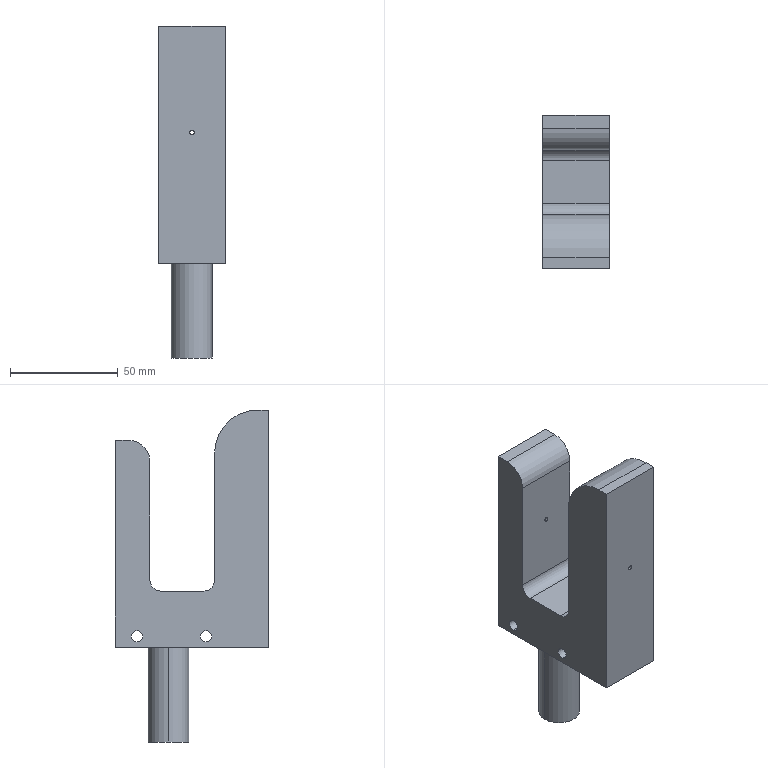Part | SolidWorks | features Fillet 3, HoleWzd 2, ICE 2, Extrusion 1 | 1 solid | 29 faces | box 31 x 71 x 154 mm | volume 164742 mm3 | cylinder 16 | plane 11 | cone 2 | commonest cylinder face diameters 2 x4 5.2 x4 5 x2 10 x2 18.868 x2 20 x1
STEP:
#1=CARTESIAN_POINT('',(5.937,16.378,-84.621));
#2=VERTEX_POINT('',#1);
#3=CARTESIAN_POINT('',(24.805,16.378,-84.621));
#4=VERTEX_POINT('',#3);
#5=CARTESIAN_POINT('',(15.371,16.378,-84.621));
#6=DIRECTION('',(0.,0.,-1.));
#7=DIRECTION('',(-1.,0.,0.));
#8=AXIS2_PLACEMENT_3D('',#5,#6,#7);
#9=CIRCLE('',#8,9.434);
#10=EDGE_CURVE('',#2,#4,#9,.T.);
#11=ORIENTED_EDGE('',*,*,#10,.F.);
#12=CARTESIAN_POINT('',(5.937,16.378,-40.621));
#13=VERTEX_POINT('',#12);
#14=CARTESIAN_POINT('',(5.937,16.378,-84.621));
#15=DIRECTION('',(0.,0.,1.));
#16=VECTOR('',#15,1000.);
#17=LINE('',#14,#16);
#18=EDGE_CURVE('',#2,#13,#17,.T.);
#19=ORIENTED_EDGE('',*,*,#18,.T.);
#20=CARTESIAN_POINT('',(24.805,16.378,-40.621));
#21=VERTEX_POINT('',#20);
#22=CARTESIAN_POINT('',(15.371,16.378,-40.621));
#23=DIRECTION('',(0.,0.,-1.));
#24=DIRECTION('',(1.,0.,0.));
#25=AXIS2_PLACEMENT_3D('',#22,#23,#24);
#26=CIRCLE('',#25,9.434);
#27=EDGE_CURVE('',#13,#21,#26,.T.);
#28=ORIENTED_EDGE('',*,*,#27,.T.);
#29=CARTESIAN_POINT('',(24.805,16.378,-84.621));
#30=DIRECTION('',(0.,0.,1.));
#31=VECTOR('',#30,1000.);
#32=LINE('',#29,#31);
#33=EDGE_CURVE('',#4,#21,#32,.T.);
#34=ORIENTED_EDGE('',*,*,#33,.F.);
#35=EDGE_LOOP('',(#11,#19,#28,#34));
#36=FACE_OUTER_BOUND('',#35,.T.);
#37=CARTESIAN_POINT('',(15.371,16.378,-84.621));
#38=DIRECTION('',(0.,0.,1.));
#39=DIRECTION('',(1.,0.,0.));
#40=AXIS2_PLACEMENT_3D('',#37,#38,#39);
#41=CYLINDRICAL_SURFACE('',#40,9.434);
#42=ADVANCED_FACE('',(#36),#41,.T.);
#43=CARTESIAN_POINT('',(18.,-13.042,-32.621));
#44=VERTEX_POINT('',#43);
#45=CARTESIAN_POINT('',(13.,-13.042,-32.621));
#46=VERTEX_POINT('',#45);
#47=CARTESIAN_POINT('',(15.5,-13.042,-32.621));
#48=DIRECTION('',(0.,0.,-1.));
#49=DIRECTION('',(-1.,0.,0.));
#50=AXIS2_PLACEMENT_3D('',#47,#48,#49);
#51=CIRCLE('',#50,2.5);
#52=EDGE_CURVE('',#44,#46,#51,.T.);
#53=ORIENTED_EDGE('',*,*,#52,.F.);
#54=CARTESIAN_POINT('',(18.,-13.042,-40.621));
#55=VERTEX_POINT('',#54);
#56=CARTESIAN_POINT('',(18.,-13.042,-40.621));
#57=DIRECTION('',(0.,0.,-1.));
#58=VECTOR('',#57,1000.);
#59=LINE('',#56,#58);
#60=EDGE_CURVE('',#44,#55,#59,.T.);
#61=ORIENTED_EDGE('',*,*,#60,.T.);
#62=CARTESIAN_POINT('',(13.,-13.042,-40.621));
#63=VERTEX_POINT('',#62);
#64=CARTESIAN_POINT('',(15.5,-13.042,-40.621));
#65=DIRECTION('',(0.,0.,-1.));
#66=DIRECTION('',(-1.,0.,0.));
#67=AXIS2_PLACEMENT_3D('',#64,#65,#66);
#68=CIRCLE('',#67,2.5);
#69=EDGE_CURVE('',#55,#63,#68,.T.);
#70=ORIENTED_EDGE('',*,*,#69,.T.);
#71=CARTESIAN_POINT('',(13.,-13.042,-40.621));
#72=DIRECTION('',(0.,0.,-1.));
#73=VECTOR('',#72,1000.);
#74=LINE('',#71,#73);
#75=EDGE_CURVE('',#46,#63,#74,.T.);
#76=ORIENTED_EDGE('',*,*,#75,.F.);
#77=EDGE_LOOP('',(#53,#61,#70,#76));
#78=FACE_OUTER_BOUND('',#77,.T.);
#79=CARTESIAN_POINT('',(15.5,-13.042,-40.621));
#80=DIRECTION('',(0.,0.,-1.));
#81=DIRECTION('',(-1.,0.,0.));
#82=AXIS2_PLACEMENT_3D('',#79,#80,#81);
#83=CYLINDRICAL_SURFACE('',#82,2.5);
#84=ADVANCED_FACE('',(#78),#83,.F.);
#85=CARTESIAN_POINT('',(15.5,-13.042,-31.119));
#86=VERTEX_POINT('',#85);
#87=CARTESIAN_POINT('',(13.,-13.042,-32.621));
#88=DIRECTION('',(-0.8572,0.,-0.515));
#89=VECTOR('',#88,1000.);
#90=LINE('',#87,#89);
#91=EDGE_CURVE('',#86,#46,#90,.T.);
#92=ORIENTED_EDGE('',*,*,#91,.F.);
#93=CARTESIAN_POINT('',(18.,-13.042,-32.621));
#94=DIRECTION('',(0.8572,0.,-0.515));
#95=VECTOR('',#94,1000.);
#96=LINE('',#93,#95);
#97=EDGE_CURVE('',#86,#44,#96,.T.);
#98=ORIENTED_EDGE('',*,*,#97,.T.);
#99=ORIENTED_EDGE('',*,*,#52,.T.);
#100=EDGE_LOOP('',(#92,#98,#99));
#101=FACE_OUTER_BOUND('',#100,.T.);
#102=CARTESIAN_POINT('',(15.5,-13.042,-32.621));
#103=DIRECTION('',(0.,0.,-1.));
#104=DIRECTION('',(-1.,0.,0.));
#105=AXIS2_PLACEMENT_3D('',#102,#103,#104);
#106=CONICAL_SURFACE('',#105,2.5,1.03);
#107=ADVANCED_FACE('',(#101),#106,.F.);
#108=CARTESIAN_POINT('',(0.,30.958,-33.021));
#109=VERTEX_POINT('',#108);
#110=CARTESIAN_POINT('',(0.,30.958,-38.221));
#111=VERTEX_POINT('',#110);
#112=CARTESIAN_POINT('',(0.,30.958,-35.621));
#113=DIRECTION('',(1.,0.,0.));
#114=DIRECTION('',(0.,0.,-1.));
#115=AXIS2_PLACEMENT_3D('',#112,#113,#114);
#116=CIRCLE('',#115,2.6);
#117=EDGE_CURVE('',#109,#111,#116,.T.);
#118=ORIENTED_EDGE('',*,*,#117,.F.);
#119=CARTESIAN_POINT('',(31.,30.958,-33.021));
#120=VERTEX_POINT('',#119);
#121=CARTESIAN_POINT('',(31.,30.958,-33.021));
#122=DIRECTION('',(1.,0.,0.));
#123=VECTOR('',#122,1000.);
#124=LINE('',#121,#123);
#125=EDGE_CURVE('',#109,#120,#124,.T.);
#126=ORIENTED_EDGE('',*,*,#125,.T.);
#127=CARTESIAN_POINT('',(31.,30.958,-38.221));
#128=VERTEX_POINT('',#127);
#129=CARTESIAN_POINT('',(31.,30.958,-35.621));
#130=DIRECTION('',(1.,0.,0.));
#131=DIRECTION('',(0.,0.,-1.));
#132=AXIS2_PLACEMENT_3D('',#129,#130,#131);
#133=CIRCLE('',#132,2.6);
#134=EDGE_CURVE('',#120,#128,#133,.T.);
#135=ORIENTED_EDGE('',*,*,#134,.T.);
#136=CARTESIAN_POINT('',(31.,30.958,-38.221));
#137=DIRECTION('',(1.,0.,0.));
#138=VECTOR('',#137,1000.);
#139=LINE('',#136,#138);
#140=EDGE_CURVE('',#111,#128,#139,.T.);
#141=ORIENTED_EDGE('',*,*,#140,.F.);
#142=EDGE_LOOP('',(#118,#126,#135,#141));
#143=FACE_OUTER_BOUND('',#142,.T.);
#144=CARTESIAN_POINT('',(31.,30.958,-35.621));
#145=DIRECTION('',(1.,0.,0.));
#146=DIRECTION('',(0.,0.,-1.));
#147=AXIS2_PLACEMENT_3D('',#144,#145,#146);
#148=CYLINDRICAL_SURFACE('',#147,2.6);
#149=ADVANCED_FACE('',(#143),#148,.F.);
#150=CARTESIAN_POINT('',(0.,-1.042,-33.021));
#151=VERTEX_POINT('',#150);
#152=CARTESIAN_POINT('',(0.,-1.042,-38.221));
#153=VERTEX_POINT('',#152);
#154=CARTESIAN_POINT('',(0.,-1.042,-35.621));
#155=DIRECTION('',(1.,0.,0.));
#156=DIRECTION('',(0.,0.,-1.));
#157=AXIS2_PLACEMENT_3D('',#154,#155,#156);
#158=CIRCLE('',#157,2.6);
#159=EDGE_CURVE('',#151,#153,#158,.T.);
#160=ORIENTED_EDGE('',*,*,#159,.F.);
#161=CARTESIAN_POINT('',(31.,-1.042,-33.021));
#162=VERTEX_POINT('',#161);
#163=CARTESIAN_POINT('',(31.,-1.042,-33.021));
#164=DIRECTION('',(1.,0.,0.));
#165=VECTOR('',#164,1000.);
#166=LINE('',#163,#165);
#167=EDGE_CURVE('',#151,#162,#166,.T.);
#168=ORIENTED_EDGE('',*,*,#167,.T.);
#169=CARTESIAN_POINT('',(31.,-1.042,-38.221));
#170=VERTEX_POINT('',#169);
#171=CARTESIAN_POINT('',(31.,-1.042,-35.621));
#172=DIRECTION('',(1.,0.,0.));
#173=DIRECTION('',(0.,0.,-1.));
#174=AXIS2_PLACEMENT_3D('',#171,#172,#173);
#175=CIRCLE('',#174,2.6);
#176=EDGE_CURVE('',#162,#170,#175,.T.);
#177=ORIENTED_EDGE('',*,*,#176,.T.);
#178=CARTESIAN_POINT('',(31.,-1.042,-38.221));
#179=DIRECTION('',(1.,0.,0.));
#180=VECTOR('',#179,1000.);
#181=LINE('',#178,#180);
#182=EDGE_CURVE('',#153,#170,#181,.T.);
#183=ORIENTED_EDGE('',*,*,#182,.F.);
#184=EDGE_LOOP('',(#160,#168,#177,#183));
#185=FACE_OUTER_BOUND('',#184,.T.);
#186=CARTESIAN_POINT('',(31.,-1.042,-35.621));
#187=DIRECTION('',(1.,0.,0.));
#188=DIRECTION('',(0.,0.,-1.));
#189=AXIS2_PLACEMENT_3D('',#186,#187,#188);
#190=CYLINDRICAL_SURFACE('',#189,2.6);
#191=ADVANCED_FACE('',(#185),#190,.F.);
#192=CARTESIAN_POINT('',(15.5,24.958,18.879));
#193=VERTEX_POINT('',#192);
#194=CARTESIAN_POINT('',(15.5,24.958,20.879));
#195=VERTEX_POINT('',#194);
#196=CARTESIAN_POINT('',(15.5,24.958,19.879));
#197=DIRECTION('',(0.,1.,0.));
#198=DIRECTION('',(0.,0.,1.));
#199=AXIS2_PLACEMENT_3D('',#196,#197,#198);
#200=CIRCLE('',#199,1.);
#201=EDGE_CURVE('',#193,#195,#200,.T.);
#202=ORIENTED_EDGE('',*,*,#201,.F.);
#203=CARTESIAN_POINT('',(15.5,40.958,18.879));
#204=VERTEX_POINT('',#203);
#205=CARTESIAN_POINT('',(15.5,-30.042,18.879));
#206=DIRECTION('',(0.,1.,0.));
#207=VECTOR('',#206,1000.);
#208=LINE('',#205,#207);
#209=EDGE_CURVE('',#193,#204,#208,.T.);
#210=ORIENTED_EDGE('',*,*,#209,.T.);
#211=CARTESIAN_POINT('',(15.5,40.958,20.879));
#212=VERTEX_POINT('',#211);
#213=CARTESIAN_POINT('',(15.5,40.958,19.879));
#214=DIRECTION('',(0.,1.,0.));
#215=DIRECTION('',(0.,0.,1.));
#216=AXIS2_PLACEMENT_3D('',#213,#214,#215);
#217=CIRCLE('',#216,1.);
#218=EDGE_CURVE('',#204,#212,#217,.T.);
#219=ORIENTED_EDGE('',*,*,#218,.T.);
#220=CARTESIAN_POINT('',(15.5,-30.042,20.879));
#221=DIRECTION('',(0.,1.,0.));
#222=VECTOR('',#221,1000.);
#223=LINE('',#220,#222);
#224=EDGE_CURVE('',#195,#212,#223,.T.);
#225=ORIENTED_EDGE('',*,*,#224,.F.);
#226=EDGE_LOOP('',(#202,#210,#219,#225));
#227=FACE_OUTER_BOUND('',#226,.T.);
#228=CARTESIAN_POINT('',(15.5,-30.042,19.879));
#229=DIRECTION('',(0.,1.,0.));
#230=DIRECTION('',(0.,0.,1.));
#231=AXIS2_PLACEMENT_3D('',#228,#229,#230);
#232=CYLINDRICAL_SURFACE('',#231,1.);
#233=ADVANCED_FACE('',(#227),#232,.F.);
#234=CARTESIAN_POINT('',(15.5,-30.042,18.879));
#235=VERTEX_POINT('',#234);
#236=CARTESIAN_POINT('',(15.5,-30.042,20.879));
#237=VERTEX_POINT('',#236);
#238=CARTESIAN_POINT('',(15.5,-30.042,19.879));
#239=DIRECTION('',(0.,1.,0.));
#240=DIRECTION('',(0.,0.,1.));
#241=AXIS2_PLACEMENT_3D('',#238,#239,#240);
#242=CIRCLE('',#241,1.);
#243=EDGE_CURVE('',#235,#237,#242,.T.);
#244=ORIENTED_EDGE('',*,*,#243,.F.);
#245=CARTESIAN_POINT('',(15.5,-5.042,18.879));
#246=VERTEX_POINT('',#245);
#247=CARTESIAN_POINT('',(15.5,-30.042,18.879));
#248=DIRECTION('',(0.,1.,0.));
#249=VECTOR('',#248,1000.);
#250=LINE('',#247,#249);
#251=EDGE_CURVE('',#235,#246,#250,.T.);
#252=ORIENTED_EDGE('',*,*,#251,.T.);
#253=CARTESIAN_POINT('',(15.5,-5.042,20.879));
#254=VERTEX_POINT('',#253);
#255=CARTESIAN_POINT('',(15.5,-5.042,19.879));
#256=DIRECTION('',(0.,-1.,0.));
#257=DIRECTION('',(0.,0.,-1.));
#258=AXIS2_PLACEMENT_3D('',#255,#256,#257);
#259=CIRCLE('',#258,1.);
#260=EDGE_CURVE('',#254,#246,#259,.T.);
#261=ORIENTED_EDGE('',*,*,#260,.F.);
#262=CARTESIAN_POINT('',(15.5,-30.042,20.879));
#263=DIRECTION('',(0.,1.,0.));
#264=VECTOR('',#263,1000.);
#265=LINE('',#262,#264);
#266=EDGE_CURVE('',#237,#254,#265,.T.);
#267=ORIENTED_EDGE('',*,*,#266,.F.);
#268=EDGE_LOOP('',(#244,#252,#261,#267));
#269=FACE_OUTER_BOUND('',#268,.T.);
#270=CARTESIAN_POINT('',(15.5,-30.042,19.879));
#271=DIRECTION('',(0.,1.,0.));
#272=DIRECTION('',(0.,0.,1.));
#273=AXIS2_PLACEMENT_3D('',#270,#271,#272);
#274=CYLINDRICAL_SURFACE('',#273,1.);
#275=ADVANCED_FACE('',(#269),#274,.F.);
#276=CARTESIAN_POINT('',(15.371,16.378,-40.621));
#277=DIRECTION('',(0.,0.,-1.));
#278=DIRECTION('',(1.,0.,0.));
#279=AXIS2_PLACEMENT_3D('',#276,#277,#278);
#280=CIRCLE('',#279,9.434);
#281=EDGE_CURVE('',#21,#13,#280,.T.);
#282=ORIENTED_EDGE('',*,*,#281,.F.);
#283=ORIENTED_EDGE('',*,*,#27,.F.);
#284=EDGE_LOOP('',(#282,#283));
#285=FACE_BOUND('',#284,.T.);
#286=CARTESIAN_POINT('',(15.5,-13.042,-40.621));
#287=DIRECTION('',(0.,0.,-1.));
#288=DIRECTION('',(-1.,0.,0.));
#289=AXIS2_PLACEMENT_3D('',#286,#287,#288);
#290=CIRCLE('',#289,2.5);
#291=EDGE_CURVE('',#63,#55,#290,.T.);
#292=ORIENTED_EDGE('',*,*,#291,.F.);
#293=ORIENTED_EDGE('',*,*,#69,.F.);
#294=EDGE_LOOP('',(#292,#293));
#295=FACE_BOUND('',#294,.T.);
#296=CARTESIAN_POINT('',(0.,-30.042,-40.621));
#297=VERTEX_POINT('',#296);
#298=CARTESIAN_POINT('',(0.,40.958,-40.621));
#299=VERTEX_POINT('',#298);
#300=CARTESIAN_POINT('',(0.,40.958,-40.621));
#301=DIRECTION('',(0.,1.,0.));
#302=VECTOR('',#301,1000.);
#303=LINE('',#300,#302);
#304=EDGE_CURVE('',#297,#299,#303,.T.);
#305=ORIENTED_EDGE('',*,*,#304,.T.);
#306=CARTESIAN_POINT('',(31.,40.958,-40.621));
#307=VERTEX_POINT('',#306);
#308=CARTESIAN_POINT('',(31.,40.958,-40.621));
#309=DIRECTION('',(-1.,0.,0.));
#310=VECTOR('',#309,1000.);
#311=LINE('',#308,#310);
#312=EDGE_CURVE('',#307,#299,#311,.T.);
#313=ORIENTED_EDGE('',*,*,#312,.F.);
#314=CARTESIAN_POINT('',(31.,-30.042,-40.621));
#315=VERTEX_POINT('',#314);
#316=CARTESIAN_POINT('',(31.,40.958,-40.621));
#317=DIRECTION('',(0.,1.,0.));
#318=VECTOR('',#317,1000.);
#319=LINE('',#316,#318);
#320=EDGE_CURVE('',#315,#307,#319,.T.);
#321=ORIENTED_EDGE('',*,*,#320,.F.);
#322=CARTESIAN_POINT('',(31.,-30.042,-40.621));
#323=DIRECTION('',(-1.,0.,0.));
#324=VECTOR('',#323,1000.);
#325=LINE('',#322,#324);
#326=EDGE_CURVE('',#315,#297,#325,.T.);
#327=ORIENTED_EDGE('',*,*,#326,.T.);
#328=EDGE_LOOP('',(#305,#313,#321,#327));
#329=FACE_OUTER_BOUND('',#328,.T.);
#330=CARTESIAN_POINT('',(31.,40.958,-40.621));
#331=DIRECTION('',(0.,0.,1.));
#332=DIRECTION('',(1.,0.,0.));
#333=AXIS2_PLACEMENT_3D('',#330,#331,#332);
#334=PLANE('',#333);
#335=ADVANCED_FACE('',(#285,#295,#329),#334,.F.);
#336=CARTESIAN_POINT('',(15.5,40.958,19.879));
#337=DIRECTION('',(0.,1.,0.));
#338=DIRECTION('',(0.,0.,1.));
#339=AXIS2_PLACEMENT_3D('',#336,#337,#338);
#340=CIRCLE('',#339,1.);
#341=EDGE_CURVE('',#212,#204,#340,.T.);
#342=ORIENTED_EDGE('',*,*,#341,.F.);
#343=ORIENTED_EDGE('',*,*,#218,.F.);
#344=EDGE_LOOP('',(#342,#343));
#345=FACE_BOUND('',#344,.T.);
#346=CARTESIAN_POINT('',(0.,40.958,55.379));
#347=VERTEX_POINT('',#346);
#348=CARTESIAN_POINT('',(0.,40.958,55.379));
#349=DIRECTION('',(0.,0.,1.));
#350=VECTOR('',#349,1000.);
#351=LINE('',#348,#350);
#352=EDGE_CURVE('',#299,#347,#351,.T.);
#353=ORIENTED_EDGE('',*,*,#352,.T.);
#354=CARTESIAN_POINT('',(31.,40.958,55.379));
#355=VERTEX_POINT('',#354);
#356=CARTESIAN_POINT('',(31.,40.958,55.379));
#357=DIRECTION('',(-1.,0.,0.));
#358=VECTOR('',#357,1000.);
#359=LINE('',#356,#358);
#360=EDGE_CURVE('',#355,#347,#359,.T.);
#361=ORIENTED_EDGE('',*,*,#360,.F.);
#362=CARTESIAN_POINT('',(31.,40.958,55.379));
#363=DIRECTION('',(0.,0.,1.));
#364=VECTOR('',#363,1000.);
#365=LINE('',#362,#364);
#366=EDGE_CURVE('',#307,#355,#365,.T.);
#367=ORIENTED_EDGE('',*,*,#366,.F.);
#368=ORIENTED_EDGE('',*,*,#312,.T.);
#369=EDGE_LOOP('',(#353,#361,#367,#368));
#370=FACE_OUTER_BOUND('',#369,.T.);
#371=CARTESIAN_POINT('',(31.,40.958,55.379));
#372=DIRECTION('',(0.,-1.,0.));
#373=DIRECTION('',(0.,0.,-1.));
#374=AXIS2_PLACEMENT_3D('',#371,#372,#373);
#375=PLANE('',#374);
#376=ADVANCED_FACE('',(#345,#370),#375,.F.);
#377=CARTESIAN_POINT('',(0.,34.958,55.379));
#378=VERTEX_POINT('',#377);
#379=CARTESIAN_POINT('',(0.,40.958,55.379));
#380=DIRECTION('',(0.,-1.,0.));
#381=VECTOR('',#380,1000.);
#382=LINE('',#379,#381);
#383=EDGE_CURVE('',#347,#378,#382,.T.);
#384=ORIENTED_EDGE('',*,*,#383,.T.);
#385=CARTESIAN_POINT('',(31.,34.958,55.379));
#386=VERTEX_POINT('',#385);
#387=CARTESIAN_POINT('',(31.,34.958,55.379));
#388=DIRECTION('',(1.,0.,0.));
#389=VECTOR('',#388,1000.);
#390=LINE('',#387,#389);
#391=EDGE_CURVE('',#378,#386,#390,.T.);
#392=ORIENTED_EDGE('',*,*,#391,.T.);
#393=CARTESIAN_POINT('',(31.,40.958,55.379));
#394=DIRECTION('',(0.,-1.,0.));
#395=VECTOR('',#394,1000.);
#396=LINE('',#393,#395);
#397=EDGE_CURVE('',#355,#386,#396,.T.);
#398=ORIENTED_EDGE('',*,*,#397,.F.);
#399=ORIENTED_EDGE('',*,*,#360,.T.);
#400=EDGE_LOOP('',(#384,#392,#398,#399));
#401=FACE_OUTER_BOUND('',#400,.T.);
#402=CARTESIAN_POINT('',(31.,40.958,55.379));
#403=DIRECTION('',(0.,0.,-1.));
#404=DIRECTION('',(-1.,0.,0.));
#405=AXIS2_PLACEMENT_3D('',#402,#403,#404);
#406=PLANE('',#405);
#407=ADVANCED_FACE('',(#401),#406,.F.);
#408=CARTESIAN_POINT('',(15.5,24.958,19.879));
#409=DIRECTION('',(0.,1.,0.));
#410=DIRECTION('',(0.,0.,1.));
#411=AXIS2_PLACEMENT_3D('',#408,#409,#410);
#412=CIRCLE('',#411,1.);
#413=EDGE_CURVE('',#195,#193,#412,.T.);
#414=ORIENTED_EDGE('',*,*,#413,.T.);
#415=ORIENTED_EDGE('',*,*,#201,.T.);
#416=EDGE_LOOP('',(#414,#415));
#417=FACE_BOUND('',#416,.T.);
#418=CARTESIAN_POINT('',(0.,24.958,45.379));
#419=VERTEX_POINT('',#418);
#420=CARTESIAN_POINT('',(0.,24.958,-9.621));
#421=VERTEX_POINT('',#420);
#422=CARTESIAN_POINT('',(0.,24.958,55.379));
#423=DIRECTION('',(0.,0.,-1.));
#424=VECTOR('',#423,1000.);
#425=LINE('',#422,#424);
#426=EDGE_CURVE('',#419,#421,#425,.T.);
#427=ORIENTED_EDGE('',*,*,#426,.T.);
#428=CARTESIAN_POINT('',(31.,24.958,-9.621));
#429=VERTEX_POINT('',#428);
#430=CARTESIAN_POINT('',(31.,24.958,-9.621));
#431=DIRECTION('',(1.,0.,0.));
#432=VECTOR('',#431,1000.);
#433=LINE('',#430,#432);
#434=EDGE_CURVE('',#421,#429,#433,.T.);
#435=ORIENTED_EDGE('',*,*,#434,.T.);
#436=CARTESIAN_POINT('',(31.,24.958,45.379));
#437=VERTEX_POINT('',#436);
#438=CARTESIAN_POINT('',(31.,24.958,55.379));
#439=DIRECTION('',(0.,0.,-1.));
#440=VECTOR('',#439,1000.);
#441=LINE('',#438,#440);
#442=EDGE_CURVE('',#437,#429,#441,.T.);
#443=ORIENTED_EDGE('',*,*,#442,.F.);
#444=CARTESIAN_POINT('',(31.,24.958,45.379));
#445=DIRECTION('',(-1.,0.,0.));
#446=VECTOR('',#445,1000.);
#447=LINE('',#444,#446);
#448=EDGE_CURVE('',#437,#419,#447,.T.);
#449=ORIENTED_EDGE('',*,*,#448,.T.);
#450=EDGE_LOOP('',(#427,#435,#443,#449));
#451=FACE_OUTER_BOUND('',#450,.T.);
#452=CARTESIAN_POINT('',(31.,24.958,55.379));
#453=DIRECTION('',(0.,1.,0.));
#454=DIRECTION('',(0.,0.,1.));
#455=AXIS2_PLACEMENT_3D('',#452,#453,#454);
#456=PLANE('',#455);
#457=ADVANCED_FACE('',(#417,#451),#456,.F.);
#458=CARTESIAN_POINT('',(0.,19.958,-14.621));
#459=VERTEX_POINT('',#458);
#460=CARTESIAN_POINT('',(0.,-0.04241,-14.621));
#461=VERTEX_POINT('',#460);
#462=CARTESIAN_POINT('',(0.,24.958,-14.621));
#463=DIRECTION('',(0.,-1.,0.));
#464=VECTOR('',#463,1000.);
#465=LINE('',#462,#464);
#466=EDGE_CURVE('',#459,#461,#465,.T.);
#467=ORIENTED_EDGE('',*,*,#466,.T.);
#468=CARTESIAN_POINT('',(31.,-0.04241,-14.621));
#469=VERTEX_POINT('',#468);
#470=CARTESIAN_POINT('',(31.,-0.04241,-14.621));
#471=DIRECTION('',(1.,0.,0.));
#472=VECTOR('',#471,1000.);
#473=LINE('',#470,#472);
#474=EDGE_CURVE('',#461,#469,#473,.T.);
#475=ORIENTED_EDGE('',*,*,#474,.T.);
#476=CARTESIAN_POINT('',(31.,19.958,-14.621));
#477=VERTEX_POINT('',#476);
#478=CARTESIAN_POINT('',(31.,24.958,-14.621));
#479=DIRECTION('',(0.,-1.,0.));
#480=VECTOR('',#479,1000.);
#481=LINE('',#478,#480);
#482=EDGE_CURVE('',#477,#469,#481,.T.);
#483=ORIENTED_EDGE('',*,*,#482,.F.);
#484=CARTESIAN_POINT('',(0.,19.958,-14.621));
#485=DIRECTION('',(-1.,0.,0.));
#486=VECTOR('',#485,1000.);
#487=LINE('',#484,#486);
#488=EDGE_CURVE('',#477,#459,#487,.T.);
#489=ORIENTED_EDGE('',*,*,#488,.T.);
#490=EDGE_LOOP('',(#467,#475,#483,#489));
#491=FACE_OUTER_BOUND('',#490,.T.);
#492=CARTESIAN_POINT('',(31.,24.958,-14.621));
#493=DIRECTION('',(0.,0.,-1.));
#494=DIRECTION('',(0.,1.,0.));
#495=AXIS2_PLACEMENT_3D('',#492,#493,#494);
#496=PLANE('',#495);
#497=ADVANCED_FACE('',(#491),#496,.F.);
#498=ORIENTED_EDGE('',*,*,#260,.T.);
#499=CARTESIAN_POINT('',(15.5,-5.042,19.879));
#500=DIRECTION('',(0.,-1.,0.));
#501=DIRECTION('',(0.,0.,-1.));
#502=AXIS2_PLACEMENT_3D('',#499,#500,#501);
#503=CIRCLE('',#502,1.);
#504=EDGE_CURVE('',#246,#254,#503,.T.);
#505=ORIENTED_EDGE('',*,*,#504,.T.);
#506=EDGE_LOOP('',(#498,#505));
#507=FACE_BOUND('',#506,.T.);
#508=CARTESIAN_POINT('',(31.,-5.042,-9.621));
#509=VERTEX_POINT('',#508);
#510=CARTESIAN_POINT('',(31.,-5.042,49.379));
#511=VERTEX_POINT('',#510);
#512=CARTESIAN_POINT('',(31.,-5.042,-14.621));
#513=DIRECTION('',(0.,0.,1.));
#514=VECTOR('',#513,1000.);
#515=LINE('',#512,#514);
#516=EDGE_CURVE('',#509,#511,#515,.T.);
#517=ORIENTED_EDGE('',*,*,#516,.F.);
#518=CARTESIAN_POINT('',(0.,-5.042,-9.621));
#519=VERTEX_POINT('',#518);
#520=CARTESIAN_POINT('',(0.,-5.042,-9.621));
#521=DIRECTION('',(-1.,0.,0.));
#522=VECTOR('',#521,1000.);
#523=LINE('',#520,#522);
#524=EDGE_CURVE('',#509,#519,#523,.T.);
#525=ORIENTED_EDGE('',*,*,#524,.T.);
#526=CARTESIAN_POINT('',(0.,-5.042,49.379));
#527=VERTEX_POINT('',#526);
#528=CARTESIAN_POINT('',(0.,-5.042,-14.621));
#529=DIRECTION('',(0.,0.,1.));
#530=VECTOR('',#529,1000.);
#531=LINE('',#528,#530);
#532=EDGE_CURVE('',#519,#527,#531,.T.);
#533=ORIENTED_EDGE('',*,*,#532,.T.);
#534=CARTESIAN_POINT('',(31.,-5.042,49.379));
#535=DIRECTION('',(1.,0.,0.));
#536=VECTOR('',#535,1000.);
#537=LINE('',#534,#536);
#538=EDGE_CURVE('',#527,#511,#537,.T.);
#539=ORIENTED_EDGE('',*,*,#538,.T.);
#540=EDGE_LOOP('',(#517,#525,#533,#539));
#541=FACE_OUTER_BOUND('',#540,.T.);
#542=CARTESIAN_POINT('',(31.,-5.042,-14.621));
#543=DIRECTION('',(0.,-1.,0.));
#544=DIRECTION('',(0.,0.,-1.));
#545=AXIS2_PLACEMENT_3D('',#542,#543,#544);
#546=PLANE('',#545);
#547=ADVANCED_FACE('',(#507,#541),#546,.F.);
#548=CARTESIAN_POINT('',(31.,-25.042,69.379));
#549=VERTEX_POINT('',#548);
#550=CARTESIAN_POINT('',(31.,-30.042,69.379));
#551=VERTEX_POINT('',#550);
#552=CARTESIAN_POINT('',(31.,-5.042,69.379));
#553=DIRECTION('',(0.,-1.,0.));
#554=VECTOR('',#553,1000.);
#555=LINE('',#552,#554);
#556=EDGE_CURVE('',#549,#551,#555,.T.);
#557=ORIENTED_EDGE('',*,*,#556,.F.);
#558=CARTESIAN_POINT('',(0.,-25.042,69.379));
#559=VERTEX_POINT('',#558);
#560=CARTESIAN_POINT('',(31.,-25.042,69.379));
#561=DIRECTION('',(-1.,0.,0.));
#562=VECTOR('',#561,1000.);
#563=LINE('',#560,#562);
#564=EDGE_CURVE('',#549,#559,#563,.T.);
#565=ORIENTED_EDGE('',*,*,#564,.T.);
#566=CARTESIAN_POINT('',(0.,-30.042,69.379));
#567=VERTEX_POINT('',#566);
#568=CARTESIAN_POINT('',(0.,-5.042,69.379));
#569=DIRECTION('',(0.,-1.,0.));
#570=VECTOR('',#569,1000.);
#571=LINE('',#568,#570);
#572=EDGE_CURVE('',#559,#567,#571,.T.);
#573=ORIENTED_EDGE('',*,*,#572,.T.);
#574=CARTESIAN_POINT('',(31.,-30.042,69.379));
#575=DIRECTION('',(-1.,0.,0.));
#576=VECTOR('',#575,1000.);
#577=LINE('',#574,#576);
#578=EDGE_CURVE('',#551,#567,#577,.T.);
#579=ORIENTED_EDGE('',*,*,#578,.F.);
#580=EDGE_LOOP('',(#557,#565,#573,#579));
#581=FACE_OUTER_BOUND('',#580,.T.);
#582=CARTESIAN_POINT('',(31.,-5.042,69.379));
#583=DIRECTION('',(0.,0.,-1.));
#584=DIRECTION('',(-1.,0.,0.));
#585=AXIS2_PLACEMENT_3D('',#582,#583,#584);
#586=PLANE('',#585);
#587=ADVANCED_FACE('',(#581),#586,.F.);
#588=CARTESIAN_POINT('',(15.5,-30.042,19.879));
#589=DIRECTION('',(0.,1.,0.));
#590=DIRECTION('',(0.,0.,1.));
#591=AXIS2_PLACEMENT_3D('',#588,#589,#590);
#592=CIRCLE('',#591,1.);
#593=EDGE_CURVE('',#237,#235,#592,.T.);
#594=ORIENTED_EDGE('',*,*,#593,.T.);
#595=ORIENTED_EDGE('',*,*,#243,.T.);
#596=EDGE_LOOP('',(#594,#595));
#597=FACE_BOUND('',#596,.T.);
#598=CARTESIAN_POINT('',(0.,-30.042,69.379));
#599=DIRECTION('',(0.,0.,-1.));
#600=VECTOR('',#599,1000.);
#601=LINE('',#598,#600);
#602=EDGE_CURVE('',#567,#297,#601,.T.);
#603=ORIENTED_EDGE('',*,*,#602,.T.);
#604=ORIENTED_EDGE('',*,*,#326,.F.);
#605=CARTESIAN_POINT('',(31.,-30.042,69.379));
#606=DIRECTION('',(0.,0.,-1.));
#607=VECTOR('',#606,1000.);
#608=LINE('',#605,#607);
#609=EDGE_CURVE('',#551,#315,#608,.T.);
#610=ORIENTED_EDGE('',*,*,#609,.F.);
#611=ORIENTED_EDGE('',*,*,#578,.T.);
#612=EDGE_LOOP('',(#603,#604,#610,#611));
#613=FACE_OUTER_BOUND('',#612,.T.);
#614=CARTESIAN_POINT('',(31.,-30.042,69.379));
#615=DIRECTION('',(0.,1.,0.));
#616=DIRECTION('',(0.,0.,1.));
#617=AXIS2_PLACEMENT_3D('',#614,#615,#616);
#618=PLANE('',#617);
#619=ADVANCED_FACE('',(#597,#613),#618,.F.);
#620=CARTESIAN_POINT('',(31.,30.958,-35.621));
#621=DIRECTION('',(1.,0.,0.));
#622=DIRECTION('',(0.,0.,-1.));
#623=AXIS2_PLACEMENT_3D('',#620,#621,#622);
#624=CIRCLE('',#623,2.6);
#625=EDGE_CURVE('',#128,#120,#624,.T.);
#626=ORIENTED_EDGE('',*,*,#625,.F.);
#627=ORIENTED_EDGE('',*,*,#134,.F.);
#628=EDGE_LOOP('',(#626,#627));
#629=FACE_BOUND('',#628,.T.);
#630=CARTESIAN_POINT('',(31.,-1.042,-35.621));
#631=DIRECTION('',(1.,0.,0.));
#632=DIRECTION('',(0.,0.,-1.));
#633=AXIS2_PLACEMENT_3D('',#630,#631,#632);
#634=CIRCLE('',#633,2.6);
#635=EDGE_CURVE('',#170,#162,#634,.T.);
#636=ORIENTED_EDGE('',*,*,#635,.F.);
#637=ORIENTED_EDGE('',*,*,#176,.F.);
#638=EDGE_LOOP('',(#636,#637));
#639=FACE_BOUND('',#638,.T.);
#640=ORIENTED_EDGE('',*,*,#482,.T.);
#641=CARTESIAN_POINT('',(31.,-0.04241,-9.621));
#642=DIRECTION('',(-1.,0.,0.));
#643=DIRECTION('',(0.,0.,-1.));
#644=AXIS2_PLACEMENT_3D('',#641,#642,#643);
#645=CIRCLE('',#644,5.);
#646=EDGE_CURVE('',#469,#509,#645,.T.);
#647=ORIENTED_EDGE('',*,*,#646,.T.);
#648=ORIENTED_EDGE('',*,*,#516,.T.);
#649=CARTESIAN_POINT('',(31.,-25.042,49.379));
#650=DIRECTION('',(1.,0.,0.));
#651=DIRECTION('',(0.,0.,-1.));
#652=AXIS2_PLACEMENT_3D('',#649,#650,#651);
#653=CIRCLE('',#652,20.);
#654=EDGE_CURVE('',#511,#549,#653,.T.);
#655=ORIENTED_EDGE('',*,*,#654,.T.);
#656=ORIENTED_EDGE('',*,*,#556,.T.);
#657=ORIENTED_EDGE('',*,*,#609,.T.);
#658=ORIENTED_EDGE('',*,*,#320,.T.);
#659=ORIENTED_EDGE('',*,*,#366,.T.);
#660=ORIENTED_EDGE('',*,*,#397,.T.);
#661=CARTESIAN_POINT('',(31.,34.958,45.379));
#662=DIRECTION('',(1.,0.,0.));
#663=DIRECTION('',(0.,0.,-1.));
#664=AXIS2_PLACEMENT_3D('',#661,#662,#663);
#665=CIRCLE('',#664,10.);
#666=EDGE_CURVE('',#386,#437,#665,.T.);
#667=ORIENTED_EDGE('',*,*,#666,.T.);
#668=ORIENTED_EDGE('',*,*,#442,.T.);
#669=CARTESIAN_POINT('',(31.,19.958,-9.621));
#670=DIRECTION('',(-1.,0.,0.));
#671=DIRECTION('',(0.,0.,-1.));
#672=AXIS2_PLACEMENT_3D('',#669,#670,#671);
#673=CIRCLE('',#672,5.);
#674=EDGE_CURVE('',#429,#477,#673,.T.);
#675=ORIENTED_EDGE('',*,*,#674,.T.);
#676=EDGE_LOOP('',(#640,#647,#648,#655,#656,#657,#658,#659,#660,#667,#668,#675));
#677=FACE_OUTER_BOUND('',#676,.T.);
#678=CARTESIAN_POINT('',(31.,0.,0.));
#679=DIRECTION('',(1.,0.,0.));
#680=DIRECTION('',(0.,0.,-1.));
#681=AXIS2_PLACEMENT_3D('',#678,#679,#680);
#682=PLANE('',#681);
#683=ADVANCED_FACE('',(#629,#639,#677),#682,.T.);
#684=CARTESIAN_POINT('',(0.,30.958,-35.621));
#685=DIRECTION('',(1.,0.,0.));
#686=DIRECTION('',(0.,0.,-1.));
#687=AXIS2_PLACEMENT_3D('',#684,#685,#686);
#688=CIRCLE('',#687,2.6);
#689=EDGE_CURVE('',#111,#109,#688,.T.);
#690=ORIENTED_EDGE('',*,*,#689,.T.);
#691=ORIENTED_EDGE('',*,*,#117,.T.);
#692=EDGE_LOOP('',(#690,#691));
#693=FACE_BOUND('',#692,.T.);
#694=CARTESIAN_POINT('',(0.,-1.042,-35.621));
#695=DIRECTION('',(1.,0.,0.));
#696=DIRECTION('',(0.,0.,-1.));
#697=AXIS2_PLACEMENT_3D('',#694,#695,#696);
#698=CIRCLE('',#697,2.6);
#699=EDGE_CURVE('',#153,#151,#698,.T.);
#700=ORIENTED_EDGE('',*,*,#699,.T.);
#701=ORIENTED_EDGE('',*,*,#159,.T.);
#702=EDGE_LOOP('',(#700,#701));
#703=FACE_BOUND('',#702,.T.);
#704=ORIENTED_EDGE('',*,*,#572,.F.);
#705=CARTESIAN_POINT('',(0.,-25.042,49.379));
#706=DIRECTION('',(-1.,0.,0.));
#707=DIRECTION('',(0.,0.,-1.));
#708=AXIS2_PLACEMENT_3D('',#705,#706,#707);
#709=CIRCLE('',#708,20.);
#710=EDGE_CURVE('',#559,#527,#709,.T.);
#711=ORIENTED_EDGE('',*,*,#710,.T.);
#712=ORIENTED_EDGE('',*,*,#532,.F.);
#713=CARTESIAN_POINT('',(0.,-0.04241,-9.621));
#714=DIRECTION('',(1.,0.,0.));
#715=DIRECTION('',(0.,0.,-1.));
#716=AXIS2_PLACEMENT_3D('',#713,#714,#715);
#717=CIRCLE('',#716,5.);
#718=EDGE_CURVE('',#519,#461,#717,.T.);
#719=ORIENTED_EDGE('',*,*,#718,.T.);
#720=ORIENTED_EDGE('',*,*,#466,.F.);
#721=CARTESIAN_POINT('',(0.,19.958,-9.621));
#722=DIRECTION('',(1.,0.,0.));
#723=DIRECTION('',(0.,0.,-1.));
#724=AXIS2_PLACEMENT_3D('',#721,#722,#723);
#725=CIRCLE('',#724,5.);
#726=EDGE_CURVE('',#459,#421,#725,.T.);
#727=ORIENTED_EDGE('',*,*,#726,.T.);
#728=ORIENTED_EDGE('',*,*,#426,.F.);
#729=CARTESIAN_POINT('',(0.,34.958,45.379));
#730=DIRECTION('',(-1.,0.,0.));
#731=DIRECTION('',(0.,0.,-1.));
#732=AXIS2_PLACEMENT_3D('',#729,#730,#731);
#733=CIRCLE('',#732,10.);
#734=EDGE_CURVE('',#419,#378,#733,.T.);
#735=ORIENTED_EDGE('',*,*,#734,.T.);
#736=ORIENTED_EDGE('',*,*,#383,.F.);
#737=ORIENTED_EDGE('',*,*,#352,.F.);
#738=ORIENTED_EDGE('',*,*,#304,.F.);
#739=ORIENTED_EDGE('',*,*,#602,.F.);
#740=EDGE_LOOP('',(#704,#711,#712,#719,#720,#727,#728,#735,#736,#737,#738,#739));
#741=FACE_OUTER_BOUND('',#740,.T.);
#742=CARTESIAN_POINT('',(0.,0.,0.));
#743=DIRECTION('',(1.,0.,0.));
#744=DIRECTION('',(0.,0.,-1.));
#745=AXIS2_PLACEMENT_3D('',#742,#743,#744);
#746=PLANE('',#745);
#747=ADVANCED_FACE('',(#693,#703,#741),#746,.F.);
#748=ORIENTED_EDGE('',*,*,#251,.F.);
#749=ORIENTED_EDGE('',*,*,#593,.F.);
#750=ORIENTED_EDGE('',*,*,#266,.T.);
#751=ORIENTED_EDGE('',*,*,#504,.F.);
#752=EDGE_LOOP('',(#748,#749,#750,#751));
#753=FACE_OUTER_BOUND('',#752,.T.);
#754=CARTESIAN_POINT('',(15.5,-30.042,19.879));
#755=DIRECTION('',(0.,1.,0.));
#756=DIRECTION('',(0.,0.,1.));
#757=AXIS2_PLACEMENT_3D('',#754,#755,#756);
#758=CYLINDRICAL_SURFACE('',#757,1.);
#759=ADVANCED_FACE('',(#753),#758,.F.);
#760=ORIENTED_EDGE('',*,*,#209,.F.);
#761=ORIENTED_EDGE('',*,*,#413,.F.);
#762=ORIENTED_EDGE('',*,*,#224,.T.);
#763=ORIENTED_EDGE('',*,*,#341,.T.);
#764=EDGE_LOOP('',(#760,#761,#762,#763));
#765=FACE_OUTER_BOUND('',#764,.T.);
#766=CARTESIAN_POINT('',(15.5,-30.042,19.879));
#767=DIRECTION('',(0.,1.,0.));
#768=DIRECTION('',(0.,0.,1.));
#769=AXIS2_PLACEMENT_3D('',#766,#767,#768);
#770=CYLINDRICAL_SURFACE('',#769,1.);
#771=ADVANCED_FACE('',(#765),#770,.F.);
#772=ORIENTED_EDGE('',*,*,#666,.F.);
#773=ORIENTED_EDGE('',*,*,#391,.F.);
#774=ORIENTED_EDGE('',*,*,#734,.F.);
#775=ORIENTED_EDGE('',*,*,#448,.F.);
#776=EDGE_LOOP('',(#772,#773,#774,#775));
#777=FACE_OUTER_BOUND('',#776,.T.);
#778=CARTESIAN_POINT('',(31.,34.958,45.379));
#779=DIRECTION('',(-1.,0.,0.));
#780=DIRECTION('',(0.,0.,1.));
#781=AXIS2_PLACEMENT_3D('',#778,#779,#780);
#782=CYLINDRICAL_SURFACE('',#781,10.);
#783=ADVANCED_FACE('',(#777),#782,.T.);
#784=ORIENTED_EDGE('',*,*,#654,.F.);
#785=ORIENTED_EDGE('',*,*,#538,.F.);
#786=ORIENTED_EDGE('',*,*,#710,.F.);
#787=ORIENTED_EDGE('',*,*,#564,.F.);
#788=EDGE_LOOP('',(#784,#785,#786,#787));
#789=FACE_OUTER_BOUND('',#788,.T.);
#790=CARTESIAN_POINT('',(31.,-25.042,49.379));
#791=DIRECTION('',(-1.,0.,0.));
#792=DIRECTION('',(0.,0.,1.));
#793=AXIS2_PLACEMENT_3D('',#790,#791,#792);
#794=CYLINDRICAL_SURFACE('',#793,20.);
#795=ADVANCED_FACE('',(#789),#794,.T.);
#796=ORIENTED_EDGE('',*,*,#646,.F.);
#797=ORIENTED_EDGE('',*,*,#474,.F.);
#798=ORIENTED_EDGE('',*,*,#718,.F.);
#799=ORIENTED_EDGE('',*,*,#524,.F.);
#800=EDGE_LOOP('',(#796,#797,#798,#799));
#801=FACE_OUTER_BOUND('',#800,.T.);
#802=CARTESIAN_POINT('',(31.,-0.04241,-9.621));
#803=DIRECTION('',(1.,0.,0.));
#804=DIRECTION('',(0.,0.,-1.));
#805=AXIS2_PLACEMENT_3D('',#802,#803,#804);
#806=CYLINDRICAL_SURFACE('',#805,5.);
#807=ADVANCED_FACE('',(#801),#806,.F.);
#808=ORIENTED_EDGE('',*,*,#674,.F.);
#809=ORIENTED_EDGE('',*,*,#434,.F.);
#810=ORIENTED_EDGE('',*,*,#726,.F.);
#811=ORIENTED_EDGE('',*,*,#488,.F.);
#812=EDGE_LOOP('',(#808,#809,#810,#811));
#813=FACE_OUTER_BOUND('',#812,.T.);
#814=CARTESIAN_POINT('',(31.,19.958,-9.621));
#815=DIRECTION('',(1.,0.,0.));
#816=DIRECTION('',(0.,0.,-1.));
#817=AXIS2_PLACEMENT_3D('',#814,#815,#816);
#818=CYLINDRICAL_SURFACE('',#817,5.);
#819=ADVANCED_FACE('',(#813),#818,.F.);
#820=ORIENTED_EDGE('',*,*,#167,.F.);
#821=ORIENTED_EDGE('',*,*,#699,.F.);
#822=ORIENTED_EDGE('',*,*,#182,.T.);
#823=ORIENTED_EDGE('',*,*,#635,.T.);
#824=EDGE_LOOP('',(#820,#821,#822,#823));
#825=FACE_OUTER_BOUND('',#824,.T.);
#826=CARTESIAN_POINT('',(31.,-1.042,-35.621));
#827=DIRECTION('',(1.,0.,0.));
#828=DIRECTION('',(0.,0.,-1.));
#829=AXIS2_PLACEMENT_3D('',#826,#827,#828);
#830=CYLINDRICAL_SURFACE('',#829,2.6);
#831=ADVANCED_FACE('',(#825),#830,.F.);
#832=ORIENTED_EDGE('',*,*,#125,.F.);
#833=ORIENTED_EDGE('',*,*,#689,.F.);
#834=ORIENTED_EDGE('',*,*,#140,.T.);
#835=ORIENTED_EDGE('',*,*,#625,.T.);
#836=EDGE_LOOP('',(#832,#833,#834,#835));
#837=FACE_OUTER_BOUND('',#836,.T.);
#838=CARTESIAN_POINT('',(31.,30.958,-35.621));
#839=DIRECTION('',(1.,0.,0.));
#840=DIRECTION('',(0.,0.,-1.));
#841=AXIS2_PLACEMENT_3D('',#838,#839,#840);
#842=CYLINDRICAL_SURFACE('',#841,2.6);
#843=ADVANCED_FACE('',(#837),#842,.F.);
#844=ORIENTED_EDGE('',*,*,#97,.F.);
#845=ORIENTED_EDGE('',*,*,#91,.T.);
#846=CARTESIAN_POINT('',(15.5,-13.042,-32.621));
#847=DIRECTION('',(0.,0.,-1.));
#848=DIRECTION('',(-1.,0.,0.));
#849=AXIS2_PLACEMENT_3D('',#846,#847,#848);
#850=CIRCLE('',#849,2.5);
#851=EDGE_CURVE('',#46,#44,#850,.T.);
#852=ORIENTED_EDGE('',*,*,#851,.T.);
#853=EDGE_LOOP('',(#844,#845,#852));
#854=FACE_OUTER_BOUND('',#853,.T.);
#855=CARTESIAN_POINT('',(15.5,-13.042,-32.621));
#856=DIRECTION('',(0.,0.,-1.));
#857=DIRECTION('',(-1.,0.,0.));
#858=AXIS2_PLACEMENT_3D('',#855,#856,#857);
#859=CONICAL_SURFACE('',#858,2.5,1.03);
#860=ADVANCED_FACE('',(#854),#859,.F.);
#861=ORIENTED_EDGE('',*,*,#60,.F.);
#862=ORIENTED_EDGE('',*,*,#851,.F.);
#863=ORIENTED_EDGE('',*,*,#75,.T.);
#864=ORIENTED_EDGE('',*,*,#291,.T.);
#865=EDGE_LOOP('',(#861,#862,#863,#864));
#866=FACE_OUTER_BOUND('',#865,.T.);
#867=CARTESIAN_POINT('',(15.5,-13.042,-40.621));
#868=DIRECTION('',(0.,0.,-1.));
#869=DIRECTION('',(-1.,0.,0.));
#870=AXIS2_PLACEMENT_3D('',#867,#868,#869);
#871=CYLINDRICAL_SURFACE('',#870,2.5);
#872=ADVANCED_FACE('',(#866),#871,.F.);
#873=ORIENTED_EDGE('',*,*,#18,.F.);
#874=CARTESIAN_POINT('',(15.371,16.378,-84.621));
#875=DIRECTION('',(0.,0.,-1.));
#876=DIRECTION('',(-1.,0.,0.));
#877=AXIS2_PLACEMENT_3D('',#874,#875,#876);
#878=CIRCLE('',#877,9.434);
#879=EDGE_CURVE('',#4,#2,#878,.T.);
#880=ORIENTED_EDGE('',*,*,#879,.F.);
#881=ORIENTED_EDGE('',*,*,#33,.T.);
#882=ORIENTED_EDGE('',*,*,#281,.T.);
#883=EDGE_LOOP('',(#873,#880,#881,#882));
#884=FACE_OUTER_BOUND('',#883,.T.);
#885=CARTESIAN_POINT('',(15.371,16.378,-84.621));
#886=DIRECTION('',(0.,0.,1.));
#887=DIRECTION('',(1.,0.,0.));
#888=AXIS2_PLACEMENT_3D('',#885,#886,#887);
#889=CYLINDRICAL_SURFACE('',#888,9.434);
#890=ADVANCED_FACE('',(#884),#889,.T.);
#891=ORIENTED_EDGE('',*,*,#879,.T.);
#892=ORIENTED_EDGE('',*,*,#10,.T.);
#893=EDGE_LOOP('',(#891,#892));
#894=FACE_OUTER_BOUND('',#893,.T.);
#895=CARTESIAN_POINT('',(15.371,16.378,-84.621));
#896=DIRECTION('',(0.,0.,-1.));
#897=DIRECTION('',(-1.,0.,0.));
#898=AXIS2_PLACEMENT_3D('',#895,#896,#897);
#899=PLANE('',#898);
#900=ADVANCED_FACE('',(#894),#899,.T.);
#901=CLOSED_SHELL('',(#42,#84,#107,#149,#191,#233,#275,#335,#376,#407,#457,#497,#547,#587,#619,#683,#747,#759,#771,#783,#795,#807,#819,#831,#843,#860,#872,#890,#900));
#902=MANIFOLD_SOLID_BREP('',#901);
#903=CARTESIAN_POINT('',(0.,0.,0.));
#904=DIRECTION('',(0.,0.,1.));
#905=DIRECTION('',(1.,0.,0.));
#906=AXIS2_PLACEMENT_3D('',#903,#904,#905);
#907=(LENGTH_UNIT()NAMED_UNIT(*)SI_UNIT(.MILLI.,.METRE.));
#908=UNCERTAINTY_MEASURE_WITH_UNIT(LENGTH_MEASURE(0.00001),#907,'','');
#909=(NAMED_UNIT(*)PLANE_ANGLE_UNIT()SI_UNIT($,.RADIAN.));
#910=(NAMED_UNIT(*)SI_UNIT($,.STERADIAN.)SOLID_ANGLE_UNIT());
#911=(GEOMETRIC_REPRESENTATION_CONTEXT(3)GLOBAL_UNCERTAINTY_ASSIGNED_CONTEXT((#908))GLOBAL_UNIT_ASSIGNED_CONTEXT((#907,#909,#910))REPRESENTATION_CONTEXT('',''));
#912=ADVANCED_BREP_SHAPE_REPRESENTATION('',(#902,#906),#911);